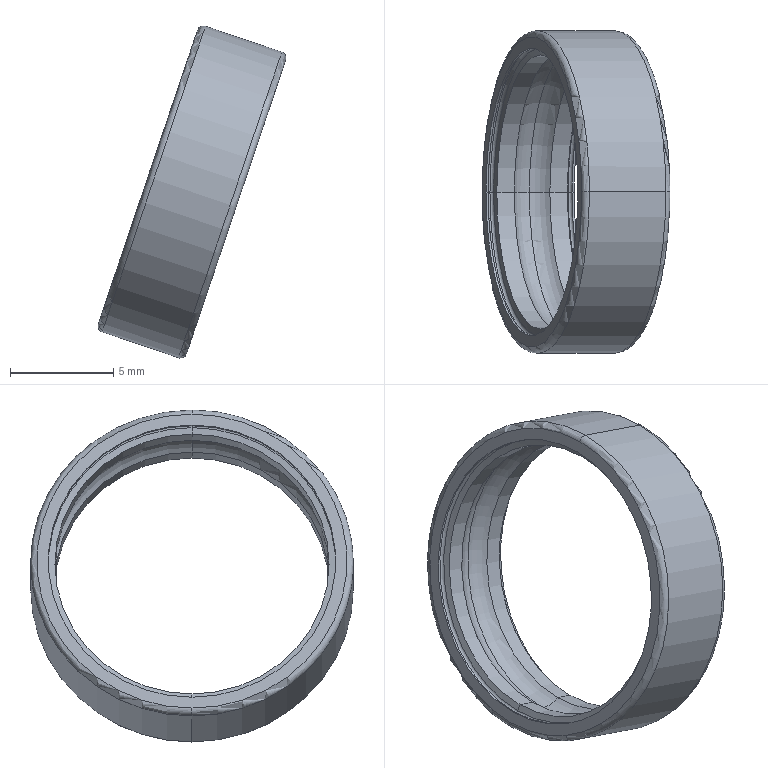Part | STEP file | 2026.6.15-Main Assembly图.sldasm-Part-183 | 1 solid | 32 faces | box 9.094 x 15.6 x 16.059 mm | volume 200.393 mm3 | torus 16 | cylinder 10 | cone 4 | plane 2 | commonest cylinder face diameters 13.26 x4 13.89 x4 15.6 x2
STEP:
#1=CARTESIAN_POINT('',(-1651.759,1424.264,3250.576));
#2=VERTEX_POINT('',#1);
#3=CARTESIAN_POINT('',(-1652.483,1424.264,3251.26));
#4=VERTEX_POINT('',#3);
#5=CARTESIAN_POINT('',(-1652.864,1424.264,3250.132));
#6=DIRECTION('',(0.,-1.,0.));
#7=DIRECTION('',(0.3199,0.,0.9474));
#8=AXIS2_PLACEMENT_3D('',#5,#6,#7);
#9=CIRCLE('',#8,1.191);
#10=EDGE_CURVE('',#2,#4,#9,.T.);
#11=ORIENTED_EDGE('',*,*,#10,.F.);
#12=CARTESIAN_POINT('',(-1656.002,1424.264,3238.013));
#13=VERTEX_POINT('',#12);
#14=CARTESIAN_POINT('',(-1653.88,1424.264,3244.295));
#15=DIRECTION('',(0.9474,0.,-0.3199));
#16=DIRECTION('',(-0.3199,0.,-0.9474));
#17=AXIS2_PLACEMENT_3D('',#14,#15,#16);
#18=CIRCLE('',#17,6.63);
#19=EDGE_CURVE('',#2,#13,#18,.T.);
#20=ORIENTED_EDGE('',*,*,#19,.T.);
#21=CARTESIAN_POINT('',(-1656.992,1424.264,3237.908));
#22=VERTEX_POINT('',#21);
#23=CARTESIAN_POINT('',(-1656.611,1424.264,3239.036));
#24=DIRECTION('',(0.,1.,0.));
#25=DIRECTION('',(-0.3199,0.,-0.9474));
#26=AXIS2_PLACEMENT_3D('',#23,#24,#25);
#27=CIRCLE('',#26,1.191);
#28=EDGE_CURVE('',#13,#22,#27,.T.);
#29=ORIENTED_EDGE('',*,*,#28,.T.);
#30=CARTESIAN_POINT('',(-1654.738,1424.264,3244.584));
#31=DIRECTION('',(0.9474,0.,-0.3199));
#32=DIRECTION('',(-0.3199,0.,-0.9474));
#33=AXIS2_PLACEMENT_3D('',#30,#31,#32);
#34=CIRCLE('',#33,7.047);
#35=EDGE_CURVE('',#4,#22,#34,.T.);
#36=ORIENTED_EDGE('',*,*,#35,.F.);
#37=EDGE_LOOP('',(#11,#20,#29,#36));
#38=FACE_OUTER_BOUND('',#37,.T.);
#39=CARTESIAN_POINT('',(-1654.738,1424.264,3244.584));
#40=DIRECTION('',(0.9474,0.,-0.3199));
#41=DIRECTION('',(-0.3199,0.,-0.9474));
#42=AXIS2_PLACEMENT_3D('',#39,#40,#41);
#43=TOROIDAL_SURFACE('',#42,5.856,1.191);
#44=ADVANCED_FACE('',(#38),#43,.F.);
#45=CARTESIAN_POINT('',(-1654.324,1424.264,3251.442));
#46=VERTEX_POINT('',#45);
#47=CARTESIAN_POINT('',(-1653.474,1424.264,3251.155));
#48=VERTEX_POINT('',#47);
#49=CARTESIAN_POINT('',(-1650.769,1424.264,3250.242));
#50=DIRECTION('',(0.9474,0.,-0.3199));
#51=VECTOR('',#50,1000.);
#52=LINE('',#49,#51);
#53=EDGE_CURVE('',#46,#48,#52,.T.);
#54=ORIENTED_EDGE('',*,*,#53,.F.);
#55=CARTESIAN_POINT('',(-1658.566,1424.264,3238.879));
#56=VERTEX_POINT('',#55);
#57=CARTESIAN_POINT('',(-1656.445,1424.264,3245.161));
#58=DIRECTION('',(-0.9474,0.,0.3199));
#59=DIRECTION('',(0.3199,0.,0.9474));
#60=AXIS2_PLACEMENT_3D('',#57,#58,#59);
#61=CIRCLE('',#60,6.63);
#62=EDGE_CURVE('',#46,#56,#61,.T.);
#63=ORIENTED_EDGE('',*,*,#62,.T.);
#64=CARTESIAN_POINT('',(-1657.716,1424.264,3238.592));
#65=VERTEX_POINT('',#64);
#66=CARTESIAN_POINT('',(-1655.011,1424.264,3237.679));
#67=DIRECTION('',(0.9474,0.,-0.3199));
#68=VECTOR('',#67,1000.);
#69=LINE('',#66,#68);
#70=EDGE_CURVE('',#56,#65,#69,.T.);
#71=ORIENTED_EDGE('',*,*,#70,.T.);
#72=CARTESIAN_POINT('',(-1655.595,1424.264,3244.873));
#73=DIRECTION('',(-0.9474,0.,0.3199));
#74=DIRECTION('',(-0.3199,0.,-0.9474));
#75=AXIS2_PLACEMENT_3D('',#72,#73,#74);
#76=CIRCLE('',#75,6.63);
#77=EDGE_CURVE('',#48,#65,#76,.T.);
#78=ORIENTED_EDGE('',*,*,#77,.F.);
#79=EDGE_LOOP('',(#54,#63,#71,#78));
#80=FACE_OUTER_BOUND('',#79,.T.);
#81=CARTESIAN_POINT('',(-1652.89,1424.264,3243.96));
#82=DIRECTION('',(0.9474,0.,-0.3199));
#83=DIRECTION('',(0.3199,0.,0.9474));
#84=AXIS2_PLACEMENT_3D('',#81,#82,#83);
#85=CYLINDRICAL_SURFACE('',#84,6.63);
#86=ADVANCED_FACE('',(#80),#85,.F.);
#87=CARTESIAN_POINT('',(-1650.909,1424.264,3250.289));
#88=VERTEX_POINT('',#87);
#89=CARTESIAN_POINT('',(-1650.769,1424.264,3250.242));
#90=DIRECTION('',(0.9474,0.,-0.3199));
#91=VECTOR('',#90,1000.);
#92=LINE('',#89,#91);
#93=EDGE_CURVE('',#2,#88,#92,.T.);
#94=ORIENTED_EDGE('',*,*,#93,.F.);
#95=CARTESIAN_POINT('',(-1653.88,1424.264,3244.295));
#96=DIRECTION('',(0.9474,0.,-0.3199));
#97=DIRECTION('',(-0.3199,0.,-0.9474));
#98=AXIS2_PLACEMENT_3D('',#95,#96,#97);
#99=CIRCLE('',#98,6.63);
#100=EDGE_CURVE('',#13,#2,#99,.T.);
#101=ORIENTED_EDGE('',*,*,#100,.F.);
#102=CARTESIAN_POINT('',(-1655.152,1424.264,3237.726));
#103=VERTEX_POINT('',#102);
#104=CARTESIAN_POINT('',(-1655.011,1424.264,3237.679));
#105=DIRECTION('',(0.9474,0.,-0.3199));
#106=VECTOR('',#105,1000.);
#107=LINE('',#104,#106);
#108=EDGE_CURVE('',#13,#103,#107,.T.);
#109=ORIENTED_EDGE('',*,*,#108,.T.);
#110=CARTESIAN_POINT('',(-1653.03,1430.894,3244.007));
#111=VERTEX_POINT('',#110);
#112=CARTESIAN_POINT('',(-1653.03,1424.264,3244.007));
#113=DIRECTION('',(0.9474,0.,-0.3199));
#114=DIRECTION('',(-0.3199,0.,-0.9474));
#115=AXIS2_PLACEMENT_3D('',#112,#113,#114);
#116=CIRCLE('',#115,6.63);
#117=EDGE_CURVE('',#103,#111,#116,.T.);
#118=ORIENTED_EDGE('',*,*,#117,.T.);
#119=CARTESIAN_POINT('',(-1653.03,1424.264,3244.007));
#120=DIRECTION('',(0.9474,0.,-0.3199));
#121=DIRECTION('',(-0.3199,0.,-0.9474));
#122=AXIS2_PLACEMENT_3D('',#119,#120,#121);
#123=CIRCLE('',#122,6.63);
#124=EDGE_CURVE('',#111,#88,#123,.T.);
#125=ORIENTED_EDGE('',*,*,#124,.T.);
#126=EDGE_LOOP('',(#94,#101,#109,#118,#125));
#127=FACE_OUTER_BOUND('',#126,.T.);
#128=CARTESIAN_POINT('',(-1652.89,1424.264,3243.96));
#129=DIRECTION('',(0.9474,0.,-0.3199));
#130=DIRECTION('',(0.3199,0.,0.9474));
#131=AXIS2_PLACEMENT_3D('',#128,#129,#130);
#132=CYLINDRICAL_SURFACE('',#131,6.63);
#133=ADVANCED_FACE('',(#127),#132,.F.);
#134=CARTESIAN_POINT('',(-1658.719,1424.264,3238.598));
#135=VERTEX_POINT('',#134);
#136=CARTESIAN_POINT('',(-1658.719,1424.264,3238.598));
#137=DIRECTION('',(0.4796,0.,0.8775));
#138=VECTOR('',#137,1000.);
#139=LINE('',#136,#138);
#140=EDGE_CURVE('',#135,#56,#139,.T.);
#141=ORIENTED_EDGE('',*,*,#140,.T.);
#142=ORIENTED_EDGE('',*,*,#62,.F.);
#143=CARTESIAN_POINT('',(-1654.275,1424.264,3251.758));
#144=VERTEX_POINT('',#143);
#145=CARTESIAN_POINT('',(-1654.275,1424.264,3251.758));
#146=DIRECTION('',(-0.1506,0.,-0.9886));
#147=VECTOR('',#146,1000.);
#148=LINE('',#145,#147);
#149=EDGE_CURVE('',#144,#46,#148,.T.);
#150=ORIENTED_EDGE('',*,*,#149,.F.);
#151=CARTESIAN_POINT('',(-1656.497,1424.264,3245.178));
#152=DIRECTION('',(-0.9474,0.,0.3199));
#153=DIRECTION('',(-0.3199,0.,-0.9474));
#154=AXIS2_PLACEMENT_3D('',#151,#152,#153);
#155=CIRCLE('',#154,6.945);
#156=EDGE_CURVE('',#144,#135,#155,.T.);
#157=ORIENTED_EDGE('',*,*,#156,.T.);
#158=EDGE_LOOP('',(#141,#142,#150,#157));
#159=FACE_OUTER_BOUND('',#158,.T.);
#160=CARTESIAN_POINT('',(-1656.497,1424.264,3245.178));
#161=DIRECTION('',(-0.9474,0.,0.3199));
#162=DIRECTION('',(-0.3199,0.,-0.9474));
#163=AXIS2_PLACEMENT_3D('',#160,#161,#162);
#164=CONICAL_SURFACE('',#163,6.945,1.396);
#165=ADVANCED_FACE('',(#159),#164,.F.);
#166=CARTESIAN_POINT('',(-1652.978,1417.319,3243.99));
#167=VERTEX_POINT('',#166);
#168=CARTESIAN_POINT('',(-1653.03,1417.634,3244.007));
#169=VERTEX_POINT('',#168);
#170=CARTESIAN_POINT('',(-1652.978,1417.319,3243.99));
#171=DIRECTION('',(-0.1645,0.9848,0.05556));
#172=VECTOR('',#171,1000.);
#173=LINE('',#170,#172);
#174=EDGE_CURVE('',#167,#169,#173,.T.);
#175=ORIENTED_EDGE('',*,*,#174,.T.);
#176=CARTESIAN_POINT('',(-1653.03,1424.264,3244.007));
#177=DIRECTION('',(0.9474,0.,-0.3199));
#178=DIRECTION('',(-0.3199,0.,-0.9474));
#179=AXIS2_PLACEMENT_3D('',#176,#177,#178);
#180=CIRCLE('',#179,6.63);
#181=EDGE_CURVE('',#88,#169,#180,.T.);
#182=ORIENTED_EDGE('',*,*,#181,.F.);
#183=ORIENTED_EDGE('',*,*,#124,.F.);
#184=CARTESIAN_POINT('',(-1652.978,1431.209,3243.99));
#185=VERTEX_POINT('',#184);
#186=CARTESIAN_POINT('',(-1652.978,1431.209,3243.99));
#187=DIRECTION('',(-0.1645,-0.9848,0.05556));
#188=VECTOR('',#187,1000.);
#189=LINE('',#186,#188);
#190=EDGE_CURVE('',#185,#111,#189,.T.);
#191=ORIENTED_EDGE('',*,*,#190,.F.);
#192=CARTESIAN_POINT('',(-1650.756,1424.264,3250.57));
#193=VERTEX_POINT('',#192);
#194=CARTESIAN_POINT('',(-1652.978,1424.264,3243.99));
#195=DIRECTION('',(0.9474,0.,-0.3199));
#196=DIRECTION('',(-0.3199,0.,-0.9474));
#197=AXIS2_PLACEMENT_3D('',#194,#195,#196);
#198=CIRCLE('',#197,6.945);
#199=EDGE_CURVE('',#185,#193,#198,.T.);
#200=ORIENTED_EDGE('',*,*,#199,.T.);
#201=CARTESIAN_POINT('',(-1652.978,1424.264,3243.99));
#202=DIRECTION('',(0.9474,0.,-0.3199));
#203=DIRECTION('',(-0.3199,0.,-0.9474));
#204=AXIS2_PLACEMENT_3D('',#201,#202,#203);
#205=CIRCLE('',#204,6.945);
#206=EDGE_CURVE('',#193,#167,#205,.T.);
#207=ORIENTED_EDGE('',*,*,#206,.T.);
#208=EDGE_LOOP('',(#175,#182,#183,#191,#200,#207));
#209=FACE_OUTER_BOUND('',#208,.T.);
#210=CARTESIAN_POINT('',(-1652.978,1424.264,3243.99));
#211=DIRECTION('',(0.9474,0.,-0.3199));
#212=DIRECTION('',(0.,-1.,0.));
#213=AXIS2_PLACEMENT_3D('',#210,#211,#212);
#214=CONICAL_SURFACE('',#213,6.945,1.396);
#215=ADVANCED_FACE('',(#209),#214,.F.);
#216=CARTESIAN_POINT('',(-1654.364,1424.264,3251.937));
#217=VERTEX_POINT('',#216);
#218=CARTESIAN_POINT('',(-1654.409,1424.264,3251.803));
#219=DIRECTION('',(0.,-1.,0.));
#220=DIRECTION('',(0.3199,0.,0.9474));
#221=AXIS2_PLACEMENT_3D('',#218,#219,#220);
#222=CIRCLE('',#221,0.1413);
#223=EDGE_CURVE('',#144,#217,#222,.T.);
#224=ORIENTED_EDGE('',*,*,#223,.F.);
#225=CARTESIAN_POINT('',(-1656.497,1424.264,3245.178));
#226=DIRECTION('',(-0.9474,0.,0.3199));
#227=DIRECTION('',(-0.3199,0.,-0.9474));
#228=AXIS2_PLACEMENT_3D('',#225,#226,#227);
#229=CIRCLE('',#228,6.945);
#230=EDGE_CURVE('',#135,#144,#229,.T.);
#231=ORIENTED_EDGE('',*,*,#230,.F.);
#232=CARTESIAN_POINT('',(-1658.898,1424.264,3238.51));
#233=VERTEX_POINT('',#232);
#234=CARTESIAN_POINT('',(-1658.853,1424.264,3238.644));
#235=DIRECTION('',(0.,1.,0.));
#236=DIRECTION('',(-0.3199,0.,-0.9474));
#237=AXIS2_PLACEMENT_3D('',#234,#235,#236);
#238=CIRCLE('',#237,0.1413);
#239=EDGE_CURVE('',#135,#233,#238,.T.);
#240=ORIENTED_EDGE('',*,*,#239,.T.);
#241=CARTESIAN_POINT('',(-1656.631,1424.264,3245.224));
#242=DIRECTION('',(0.9474,0.,-0.3199));
#243=DIRECTION('',(-0.3199,0.,-0.9474));
#244=AXIS2_PLACEMENT_3D('',#241,#242,#243);
#245=CIRCLE('',#244,7.086);
#246=EDGE_CURVE('',#217,#233,#245,.T.);
#247=ORIENTED_EDGE('',*,*,#246,.F.);
#248=EDGE_LOOP('',(#224,#231,#240,#247));
#249=FACE_OUTER_BOUND('',#248,.T.);
#250=CARTESIAN_POINT('',(-1656.631,1424.264,3245.224));
#251=DIRECTION('',(0.9474,0.,-0.3199));
#252=DIRECTION('',(-0.3199,0.,-0.9474));
#253=AXIS2_PLACEMENT_3D('',#250,#251,#252);
#254=TOROIDAL_SURFACE('',#253,6.945,0.1413);
#255=ADVANCED_FACE('',(#249),#254,.F.);
#256=CARTESIAN_POINT('',(-1650.488,1424.264,3250.479));
#257=VERTEX_POINT('',#256);
#258=CARTESIAN_POINT('',(-1650.577,1424.264,3250.658));
#259=VERTEX_POINT('',#258);
#260=CARTESIAN_POINT('',(-1650.622,1424.264,3250.524));
#261=DIRECTION('',(0.,-1.,0.));
#262=DIRECTION('',(0.3199,0.,0.9474));
#263=AXIS2_PLACEMENT_3D('',#260,#261,#262);
#264=CIRCLE('',#263,0.1413);
#265=EDGE_CURVE('',#257,#259,#264,.T.);
#266=ORIENTED_EDGE('',*,*,#265,.F.);
#267=CARTESIAN_POINT('',(-1654.932,1424.264,3237.319));
#268=VERTEX_POINT('',#267);
#269=CARTESIAN_POINT('',(-1652.71,1424.264,3243.899));
#270=DIRECTION('',(0.9474,0.,-0.3199));
#271=DIRECTION('',(-0.3199,0.,-0.9474));
#272=AXIS2_PLACEMENT_3D('',#269,#270,#271);
#273=CIRCLE('',#272,6.945);
#274=EDGE_CURVE('',#257,#268,#273,.T.);
#275=ORIENTED_EDGE('',*,*,#274,.T.);
#276=CARTESIAN_POINT('',(-1655.111,1424.264,3237.231));
#277=VERTEX_POINT('',#276);
#278=CARTESIAN_POINT('',(-1655.066,1424.264,3237.365));
#279=DIRECTION('',(0.,1.,0.));
#280=DIRECTION('',(-0.3199,0.,-0.9474));
#281=AXIS2_PLACEMENT_3D('',#278,#279,#280);
#282=CIRCLE('',#281,0.1413);
#283=EDGE_CURVE('',#268,#277,#282,.T.);
#284=ORIENTED_EDGE('',*,*,#283,.T.);
#285=CARTESIAN_POINT('',(-1652.844,1424.264,3243.944));
#286=DIRECTION('',(0.9474,0.,-0.3199));
#287=DIRECTION('',(-0.3199,0.,-0.9474));
#288=AXIS2_PLACEMENT_3D('',#285,#286,#287);
#289=CIRCLE('',#288,7.086);
#290=EDGE_CURVE('',#259,#277,#289,.T.);
#291=ORIENTED_EDGE('',*,*,#290,.F.);
#292=EDGE_LOOP('',(#266,#275,#284,#291));
#293=FACE_OUTER_BOUND('',#292,.T.);
#294=CARTESIAN_POINT('',(-1652.844,1424.264,3243.944));
#295=DIRECTION('',(0.9474,0.,-0.3199));
#296=DIRECTION('',(-0.3199,0.,-0.9474));
#297=AXIS2_PLACEMENT_3D('',#294,#295,#296);
#298=TOROIDAL_SURFACE('',#297,6.945,0.1413);
#299=ADVANCED_FACE('',(#293),#298,.F.);
#300=CARTESIAN_POINT('',(-1654.647,1424.264,3251.884));
#301=VERTEX_POINT('',#300);
#302=CARTESIAN_POINT('',(-1654.543,1424.264,3251.849));
#303=VERTEX_POINT('',#302);
#304=CARTESIAN_POINT('',(-1650.668,1424.264,3250.54));
#305=DIRECTION('',(0.9474,0.,-0.3199));
#306=VECTOR('',#305,1000.);
#307=LINE('',#304,#306);
#308=EDGE_CURVE('',#301,#303,#307,.T.);
#309=ORIENTED_EDGE('',*,*,#308,.F.);
#310=CARTESIAN_POINT('',(-1659.091,1424.264,3238.724));
#311=VERTEX_POINT('',#310);
#312=CARTESIAN_POINT('',(-1656.869,1424.264,3245.304));
#313=DIRECTION('',(0.9474,0.,-0.3199));
#314=DIRECTION('',(-0.3199,0.,-0.9474));
#315=AXIS2_PLACEMENT_3D('',#312,#313,#314);
#316=CIRCLE('',#315,6.945);
#317=EDGE_CURVE('',#311,#301,#316,.T.);
#318=ORIENTED_EDGE('',*,*,#317,.F.);
#319=CARTESIAN_POINT('',(-1658.987,1424.264,3238.689));
#320=VERTEX_POINT('',#319);
#321=CARTESIAN_POINT('',(-1655.112,1424.264,3237.38));
#322=DIRECTION('',(0.9474,0.,-0.3199));
#323=VECTOR('',#322,1000.);
#324=LINE('',#321,#323);
#325=EDGE_CURVE('',#311,#320,#324,.T.);
#326=ORIENTED_EDGE('',*,*,#325,.T.);
#327=CARTESIAN_POINT('',(-1656.765,1424.264,3245.269));
#328=DIRECTION('',(-0.9474,0.,0.3199));
#329=DIRECTION('',(-0.3199,0.,-0.9474));
#330=AXIS2_PLACEMENT_3D('',#327,#328,#329);
#331=CIRCLE('',#330,6.945);
#332=EDGE_CURVE('',#303,#320,#331,.T.);
#333=ORIENTED_EDGE('',*,*,#332,.F.);
#334=EDGE_LOOP('',(#309,#318,#326,#333));
#335=FACE_OUTER_BOUND('',#334,.T.);
#336=CARTESIAN_POINT('',(-1652.89,1424.264,3243.96));
#337=DIRECTION('',(0.9474,0.,-0.3199));
#338=DIRECTION('',(0.3199,0.,0.9474));
#339=AXIS2_PLACEMENT_3D('',#336,#337,#338);
#340=CYLINDRICAL_SURFACE('',#339,6.945);
#341=ADVANCED_FACE('',(#335),#340,.F.);
#342=CARTESIAN_POINT('',(-1650.384,1424.264,3250.444));
#343=VERTEX_POINT('',#342);
#344=CARTESIAN_POINT('',(-1650.668,1424.264,3250.54));
#345=DIRECTION('',(0.9474,0.,-0.3199));
#346=VECTOR('',#345,1000.);
#347=LINE('',#344,#346);
#348=EDGE_CURVE('',#257,#343,#347,.T.);
#349=ORIENTED_EDGE('',*,*,#348,.F.);
#350=CARTESIAN_POINT('',(-1652.71,1424.264,3243.899));
#351=DIRECTION('',(0.9474,0.,-0.3199));
#352=DIRECTION('',(-0.3199,0.,-0.9474));
#353=AXIS2_PLACEMENT_3D('',#350,#351,#352);
#354=CIRCLE('',#353,6.945);
#355=EDGE_CURVE('',#268,#257,#354,.T.);
#356=ORIENTED_EDGE('',*,*,#355,.F.);
#357=CARTESIAN_POINT('',(-1654.828,1424.264,3237.284));
#358=VERTEX_POINT('',#357);
#359=CARTESIAN_POINT('',(-1655.112,1424.264,3237.38));
#360=DIRECTION('',(0.9474,0.,-0.3199));
#361=VECTOR('',#360,1000.);
#362=LINE('',#359,#361);
#363=EDGE_CURVE('',#268,#358,#362,.T.);
#364=ORIENTED_EDGE('',*,*,#363,.T.);
#365=CARTESIAN_POINT('',(-1652.606,1424.264,3243.864));
#366=DIRECTION('',(-0.9474,0.,0.3199));
#367=DIRECTION('',(-0.3199,0.,-0.9474));
#368=AXIS2_PLACEMENT_3D('',#365,#366,#367);
#369=CIRCLE('',#368,6.945);
#370=EDGE_CURVE('',#343,#358,#369,.T.);
#371=ORIENTED_EDGE('',*,*,#370,.F.);
#372=EDGE_LOOP('',(#349,#356,#364,#371));
#373=FACE_OUTER_BOUND('',#372,.T.);
#374=CARTESIAN_POINT('',(-1652.89,1424.264,3243.96));
#375=DIRECTION('',(0.9474,0.,-0.3199));
#376=DIRECTION('',(0.3199,0.,0.9474));
#377=AXIS2_PLACEMENT_3D('',#374,#375,#376);
#378=CYLINDRICAL_SURFACE('',#377,6.945);
#379=ADVANCED_FACE('',(#373),#378,.F.);
#380=CARTESIAN_POINT('',(-1659.269,1424.264,3238.198));
#381=VERTEX_POINT('',#380);
#382=CARTESIAN_POINT('',(-1654.47,1424.264,3252.41));
#383=VERTEX_POINT('',#382);
#384=CARTESIAN_POINT('',(-1656.869,1424.264,3245.304));
#385=DIRECTION('',(0.9474,0.,-0.3199));
#386=DIRECTION('',(-0.3199,0.,-0.9474));
#387=AXIS2_PLACEMENT_3D('',#384,#385,#386);
#388=CIRCLE('',#387,7.5);
#389=EDGE_CURVE('',#381,#383,#388,.T.);
#390=ORIENTED_EDGE('',*,*,#389,.F.);
#391=CARTESIAN_POINT('',(-1656.869,1424.264,3245.304));
#392=DIRECTION('',(0.9474,0.,-0.3199));
#393=DIRECTION('',(-0.3199,0.,-0.9474));
#394=AXIS2_PLACEMENT_3D('',#391,#392,#393);
#395=CIRCLE('',#394,7.5);
#396=EDGE_CURVE('',#383,#381,#395,.T.);
#397=ORIENTED_EDGE('',*,*,#396,.F.);
#398=EDGE_LOOP('',(#390,#397));
#399=FACE_OUTER_BOUND('',#398,.T.);
#400=ORIENTED_EDGE('',*,*,#317,.T.);
#401=CARTESIAN_POINT('',(-1656.869,1424.264,3245.304));
#402=DIRECTION('',(0.9474,0.,-0.3199));
#403=DIRECTION('',(-0.3199,0.,-0.9474));
#404=AXIS2_PLACEMENT_3D('',#401,#402,#403);
#405=CIRCLE('',#404,6.945);
#406=EDGE_CURVE('',#301,#311,#405,.T.);
#407=ORIENTED_EDGE('',*,*,#406,.T.);
#408=EDGE_LOOP('',(#400,#407));
#409=FACE_BOUND('',#408,.T.);
#410=CARTESIAN_POINT('',(-1656.869,1431.764,3245.304));
#411=DIRECTION('',(-0.9474,0.,0.3199));
#412=DIRECTION('',(0.,1.,0.));
#413=AXIS2_PLACEMENT_3D('',#410,#411,#412);
#414=PLANE('',#413);
#415=ADVANCED_FACE('',(#399,#409),#414,.T.);
#416=CARTESIAN_POINT('',(-1650.206,1424.264,3250.97));
#417=VERTEX_POINT('',#416);
#418=CARTESIAN_POINT('',(-1655.005,1424.264,3236.758));
#419=VERTEX_POINT('',#418);
#420=CARTESIAN_POINT('',(-1652.606,1424.264,3243.864));
#421=DIRECTION('',(-0.9474,0.,0.3199));
#422=DIRECTION('',(0.3199,0.,0.9474));
#423=AXIS2_PLACEMENT_3D('',#420,#421,#422);
#424=CIRCLE('',#423,7.5);
#425=EDGE_CURVE('',#417,#419,#424,.T.);
#426=ORIENTED_EDGE('',*,*,#425,.F.);
#427=CARTESIAN_POINT('',(-1652.606,1424.264,3243.864));
#428=DIRECTION('',(-0.9474,0.,0.3199));
#429=DIRECTION('',(0.3199,0.,0.9474));
#430=AXIS2_PLACEMENT_3D('',#427,#428,#429);
#431=CIRCLE('',#430,7.5);
#432=EDGE_CURVE('',#419,#417,#431,.T.);
#433=ORIENTED_EDGE('',*,*,#432,.F.);
#434=EDGE_LOOP('',(#426,#433));
#435=FACE_OUTER_BOUND('',#434,.T.);
#436=CARTESIAN_POINT('',(-1652.606,1424.264,3243.864));
#437=DIRECTION('',(-0.9474,0.,0.3199));
#438=DIRECTION('',(-0.3199,0.,-0.9474));
#439=AXIS2_PLACEMENT_3D('',#436,#437,#438);
#440=CIRCLE('',#439,6.945);
#441=EDGE_CURVE('',#358,#343,#440,.T.);
#442=ORIENTED_EDGE('',*,*,#441,.T.);
#443=ORIENTED_EDGE('',*,*,#370,.T.);
#444=EDGE_LOOP('',(#442,#443));
#445=FACE_BOUND('',#444,.T.);
#446=CARTESIAN_POINT('',(-1652.606,1431.209,3243.864));
#447=DIRECTION('',(0.9474,0.,-0.3199));
#448=DIRECTION('',(0.,-1.,0.));
#449=AXIS2_PLACEMENT_3D('',#446,#447,#448);
#450=PLANE('',#449);
#451=ADVANCED_FACE('',(#435,#445),#450,.T.);
#452=CARTESIAN_POINT('',(-1654.089,1424.264,3252.598));
#453=VERTEX_POINT('',#452);
#454=CARTESIAN_POINT('',(-1654.185,1424.264,3252.314));
#455=DIRECTION('',(0.,-1.,0.));
#456=DIRECTION('',(0.3199,0.,0.9474));
#457=AXIS2_PLACEMENT_3D('',#454,#455,#456);
#458=CIRCLE('',#457,0.3);
#459=EDGE_CURVE('',#453,#383,#458,.T.);
#460=ORIENTED_EDGE('',*,*,#459,.F.);
#461=CARTESIAN_POINT('',(-1659.081,1424.264,3237.818));
#462=VERTEX_POINT('',#461);
#463=CARTESIAN_POINT('',(-1656.585,1424.264,3245.208));
#464=DIRECTION('',(0.9474,0.,-0.3199));
#465=DIRECTION('',(-0.3199,0.,-0.9474));
#466=AXIS2_PLACEMENT_3D('',#463,#464,#465);
#467=CIRCLE('',#466,7.8);
#468=EDGE_CURVE('',#462,#453,#467,.T.);
#469=ORIENTED_EDGE('',*,*,#468,.F.);
#470=CARTESIAN_POINT('',(-1658.985,1424.264,3238.102));
#471=DIRECTION('',(0.,1.,0.));
#472=DIRECTION('',(-0.3199,0.,-0.9474));
#473=AXIS2_PLACEMENT_3D('',#470,#471,#472);
#474=CIRCLE('',#473,0.3);
#475=EDGE_CURVE('',#462,#381,#474,.T.);
#476=ORIENTED_EDGE('',*,*,#475,.T.);
#477=ORIENTED_EDGE('',*,*,#389,.T.);
#478=EDGE_LOOP('',(#460,#469,#476,#477));
#479=FACE_OUTER_BOUND('',#478,.T.);
#480=CARTESIAN_POINT('',(-1656.585,1424.264,3245.208));
#481=DIRECTION('',(0.9474,0.,-0.3199));
#482=DIRECTION('',(-0.3199,0.,-0.9474));
#483=AXIS2_PLACEMENT_3D('',#480,#481,#482);
#484=TOROIDAL_SURFACE('',#483,7.5,0.3);
#485=ADVANCED_FACE('',(#479),#484,.T.);
#486=CARTESIAN_POINT('',(-1650.394,1424.264,3251.35));
#487=VERTEX_POINT('',#486);
#488=CARTESIAN_POINT('',(-1650.49,1424.264,3251.066));
#489=DIRECTION('',(0.,-1.,0.));
#490=DIRECTION('',(0.3199,0.,0.9474));
#491=AXIS2_PLACEMENT_3D('',#488,#489,#490);
#492=CIRCLE('',#491,0.3);
#493=EDGE_CURVE('',#417,#487,#492,.T.);
#494=ORIENTED_EDGE('',*,*,#493,.F.);
#495=ORIENTED_EDGE('',*,*,#425,.T.);
#496=CARTESIAN_POINT('',(-1655.386,1424.264,3236.57));
#497=VERTEX_POINT('',#496);
#498=CARTESIAN_POINT('',(-1655.29,1424.264,3236.854));
#499=DIRECTION('',(0.,1.,0.));
#500=DIRECTION('',(-0.3199,0.,-0.9474));
#501=AXIS2_PLACEMENT_3D('',#498,#499,#500);
#502=CIRCLE('',#501,0.3);
#503=EDGE_CURVE('',#419,#497,#502,.T.);
#504=ORIENTED_EDGE('',*,*,#503,.T.);
#505=CARTESIAN_POINT('',(-1652.89,1424.264,3243.96));
#506=DIRECTION('',(-0.9474,0.,0.3199));
#507=DIRECTION('',(-0.3199,0.,-0.9474));
#508=AXIS2_PLACEMENT_3D('',#505,#506,#507);
#509=CIRCLE('',#508,7.8);
#510=EDGE_CURVE('',#487,#497,#509,.T.);
#511=ORIENTED_EDGE('',*,*,#510,.F.);
#512=EDGE_LOOP('',(#494,#495,#504,#511));
#513=FACE_OUTER_BOUND('',#512,.T.);
#514=CARTESIAN_POINT('',(-1652.89,1424.264,3243.96));
#515=DIRECTION('',(0.9474,0.,-0.3199));
#516=DIRECTION('',(-0.3199,0.,-0.9474));
#517=AXIS2_PLACEMENT_3D('',#514,#515,#516);
#518=TOROIDAL_SURFACE('',#517,7.5,0.3);
#519=ADVANCED_FACE('',(#513),#518,.T.);
#520=CARTESIAN_POINT('',(-1650.394,1424.264,3251.35));
#521=DIRECTION('',(0.9474,0.,-0.3199));
#522=VECTOR('',#521,1000.);
#523=LINE('',#520,#522);
#524=EDGE_CURVE('',#453,#487,#523,.T.);
#525=ORIENTED_EDGE('',*,*,#524,.F.);
#526=CARTESIAN_POINT('',(-1656.585,1424.264,3245.208));
#527=DIRECTION('',(0.9474,0.,-0.3199));
#528=DIRECTION('',(-0.3199,0.,-0.9474));
#529=AXIS2_PLACEMENT_3D('',#526,#527,#528);
#530=CIRCLE('',#529,7.8);
#531=EDGE_CURVE('',#453,#462,#530,.T.);
#532=ORIENTED_EDGE('',*,*,#531,.T.);
#533=CARTESIAN_POINT('',(-1655.386,1424.264,3236.57));
#534=DIRECTION('',(0.9474,0.,-0.3199));
#535=VECTOR('',#534,1000.);
#536=LINE('',#533,#535);
#537=EDGE_CURVE('',#462,#497,#536,.T.);
#538=ORIENTED_EDGE('',*,*,#537,.T.);
#539=CARTESIAN_POINT('',(-1652.89,1424.264,3243.96));
#540=DIRECTION('',(-0.9474,0.,0.3199));
#541=DIRECTION('',(-0.3199,0.,-0.9474));
#542=AXIS2_PLACEMENT_3D('',#539,#540,#541);
#543=CIRCLE('',#542,7.8);
#544=EDGE_CURVE('',#497,#487,#543,.T.);
#545=ORIENTED_EDGE('',*,*,#544,.T.);
#546=EDGE_LOOP('',(#525,#532,#538,#545));
#547=FACE_OUTER_BOUND('',#546,.T.);
#548=CARTESIAN_POINT('',(-1652.89,1424.264,3243.96));
#549=DIRECTION('',(0.9474,0.,-0.3199));
#550=DIRECTION('',(0.3199,0.,0.9474));
#551=AXIS2_PLACEMENT_3D('',#548,#549,#550);
#552=CYLINDRICAL_SURFACE('',#551,7.8);
#553=ADVANCED_FACE('',(#547),#552,.T.);
#554=CARTESIAN_POINT('',(-1652.864,1424.264,3250.132));
#555=DIRECTION('',(0.,-1.,0.));
#556=DIRECTION('',(0.3199,0.,0.9474));
#557=AXIS2_PLACEMENT_3D('',#554,#555,#556);
#558=CIRCLE('',#557,1.191);
#559=EDGE_CURVE('',#4,#48,#558,.T.);
#560=ORIENTED_EDGE('',*,*,#559,.F.);
#561=ORIENTED_EDGE('',*,*,#35,.T.);
#562=CARTESIAN_POINT('',(-1656.611,1424.264,3239.036));
#563=DIRECTION('',(0.,1.,0.));
#564=DIRECTION('',(-0.3199,0.,-0.9474));
#565=AXIS2_PLACEMENT_3D('',#562,#563,#564);
#566=CIRCLE('',#565,1.191);
#567=EDGE_CURVE('',#22,#65,#566,.T.);
#568=ORIENTED_EDGE('',*,*,#567,.T.);
#569=CARTESIAN_POINT('',(-1655.595,1424.264,3244.873));
#570=DIRECTION('',(-0.9474,0.,0.3199));
#571=DIRECTION('',(-0.3199,0.,-0.9474));
#572=AXIS2_PLACEMENT_3D('',#569,#570,#571);
#573=CIRCLE('',#572,6.63);
#574=EDGE_CURVE('',#65,#48,#573,.T.);
#575=ORIENTED_EDGE('',*,*,#574,.T.);
#576=EDGE_LOOP('',(#560,#561,#568,#575));
#577=FACE_OUTER_BOUND('',#576,.T.);
#578=CARTESIAN_POINT('',(-1654.738,1424.264,3244.584));
#579=DIRECTION('',(0.9474,0.,-0.3199));
#580=DIRECTION('',(-0.3199,0.,-0.9474));
#581=AXIS2_PLACEMENT_3D('',#578,#579,#580);
#582=TOROIDAL_SURFACE('',#581,5.856,1.191);
#583=ADVANCED_FACE('',(#577),#582,.F.);
#584=CARTESIAN_POINT('',(-1656.445,1424.264,3245.161));
#585=DIRECTION('',(-0.9474,0.,0.3199));
#586=DIRECTION('',(0.3199,0.,0.9474));
#587=AXIS2_PLACEMENT_3D('',#584,#585,#586);
#588=CIRCLE('',#587,6.63);
#589=EDGE_CURVE('',#56,#46,#588,.T.);
#590=ORIENTED_EDGE('',*,*,#589,.T.);
#591=ORIENTED_EDGE('',*,*,#53,.T.);
#592=ORIENTED_EDGE('',*,*,#574,.F.);
#593=ORIENTED_EDGE('',*,*,#70,.F.);
#594=EDGE_LOOP('',(#590,#591,#592,#593));
#595=FACE_OUTER_BOUND('',#594,.T.);
#596=CARTESIAN_POINT('',(-1652.89,1424.264,3243.96));
#597=DIRECTION('',(0.9474,0.,-0.3199));
#598=DIRECTION('',(0.3199,0.,0.9474));
#599=AXIS2_PLACEMENT_3D('',#596,#597,#598);
#600=CYLINDRICAL_SURFACE('',#599,6.63);
#601=ADVANCED_FACE('',(#595),#600,.F.);
#602=ORIENTED_EDGE('',*,*,#19,.F.);
#603=ORIENTED_EDGE('',*,*,#93,.T.);
#604=ORIENTED_EDGE('',*,*,#181,.T.);
#605=CARTESIAN_POINT('',(-1653.03,1424.264,3244.007));
#606=DIRECTION('',(0.9474,0.,-0.3199));
#607=DIRECTION('',(-0.3199,0.,-0.9474));
#608=AXIS2_PLACEMENT_3D('',#605,#606,#607);
#609=CIRCLE('',#608,6.63);
#610=EDGE_CURVE('',#169,#103,#609,.T.);
#611=ORIENTED_EDGE('',*,*,#610,.T.);
#612=ORIENTED_EDGE('',*,*,#108,.F.);
#613=EDGE_LOOP('',(#602,#603,#604,#611,#612));
#614=FACE_OUTER_BOUND('',#613,.T.);
#615=CARTESIAN_POINT('',(-1652.89,1424.264,3243.96));
#616=DIRECTION('',(0.9474,0.,-0.3199));
#617=DIRECTION('',(0.3199,0.,0.9474));
#618=AXIS2_PLACEMENT_3D('',#615,#616,#617);
#619=CYLINDRICAL_SURFACE('',#618,6.63);
#620=ADVANCED_FACE('',(#614),#619,.F.);
#621=ORIENTED_EDGE('',*,*,#589,.F.);
#622=ORIENTED_EDGE('',*,*,#140,.F.);
#623=ORIENTED_EDGE('',*,*,#230,.T.);
#624=ORIENTED_EDGE('',*,*,#149,.T.);
#625=EDGE_LOOP('',(#621,#622,#623,#624));
#626=FACE_OUTER_BOUND('',#625,.T.);
#627=CARTESIAN_POINT('',(-1656.497,1424.264,3245.178));
#628=DIRECTION('',(-0.9474,0.,0.3199));
#629=DIRECTION('',(-0.3199,0.,-0.9474));
#630=AXIS2_PLACEMENT_3D('',#627,#628,#629);
#631=CONICAL_SURFACE('',#630,6.945,1.396);
#632=ADVANCED_FACE('',(#626),#631,.F.);
#633=ORIENTED_EDGE('',*,*,#610,.F.);
#634=ORIENTED_EDGE('',*,*,#174,.F.);
#635=CARTESIAN_POINT('',(-1655.2,1424.264,3237.41));
#636=VERTEX_POINT('',#635);
#637=CARTESIAN_POINT('',(-1652.978,1424.264,3243.99));
#638=DIRECTION('',(0.9474,0.,-0.3199));
#639=DIRECTION('',(-0.3199,0.,-0.9474));
#640=AXIS2_PLACEMENT_3D('',#637,#638,#639);
#641=CIRCLE('',#640,6.945);
#642=EDGE_CURVE('',#167,#636,#641,.T.);
#643=ORIENTED_EDGE('',*,*,#642,.T.);
#644=CARTESIAN_POINT('',(-1652.978,1424.264,3243.99));
#645=DIRECTION('',(0.9474,0.,-0.3199));
#646=DIRECTION('',(-0.3199,0.,-0.9474));
#647=AXIS2_PLACEMENT_3D('',#644,#645,#646);
#648=CIRCLE('',#647,6.945);
#649=EDGE_CURVE('',#636,#185,#648,.T.);
#650=ORIENTED_EDGE('',*,*,#649,.T.);
#651=ORIENTED_EDGE('',*,*,#190,.T.);
#652=ORIENTED_EDGE('',*,*,#117,.F.);
#653=EDGE_LOOP('',(#633,#634,#643,#650,#651,#652));
#654=FACE_OUTER_BOUND('',#653,.T.);
#655=CARTESIAN_POINT('',(-1652.978,1424.264,3243.99));
#656=DIRECTION('',(0.9474,0.,-0.3199));
#657=DIRECTION('',(0.,-1.,0.));
#658=AXIS2_PLACEMENT_3D('',#655,#656,#657);
#659=CONICAL_SURFACE('',#658,6.945,1.396);
#660=ADVANCED_FACE('',(#654),#659,.F.);
#661=CARTESIAN_POINT('',(-1654.409,1424.264,3251.803));
#662=DIRECTION('',(0.,-1.,0.));
#663=DIRECTION('',(0.3199,0.,0.9474));
#664=AXIS2_PLACEMENT_3D('',#661,#662,#663);
#665=CIRCLE('',#664,0.1413);
#666=EDGE_CURVE('',#217,#303,#665,.T.);
#667=ORIENTED_EDGE('',*,*,#666,.F.);
#668=ORIENTED_EDGE('',*,*,#246,.T.);
#669=CARTESIAN_POINT('',(-1658.853,1424.264,3238.644));
#670=DIRECTION('',(0.,1.,0.));
#671=DIRECTION('',(-0.3199,0.,-0.9474));
#672=AXIS2_PLACEMENT_3D('',#669,#670,#671);
#673=CIRCLE('',#672,0.1413);
#674=EDGE_CURVE('',#233,#320,#673,.T.);
#675=ORIENTED_EDGE('',*,*,#674,.T.);
#676=CARTESIAN_POINT('',(-1656.765,1424.264,3245.269));
#677=DIRECTION('',(-0.9474,0.,0.3199));
#678=DIRECTION('',(-0.3199,0.,-0.9474));
#679=AXIS2_PLACEMENT_3D('',#676,#677,#678);
#680=CIRCLE('',#679,6.945);
#681=EDGE_CURVE('',#320,#303,#680,.T.);
#682=ORIENTED_EDGE('',*,*,#681,.T.);
#683=EDGE_LOOP('',(#667,#668,#675,#682));
#684=FACE_OUTER_BOUND('',#683,.T.);
#685=CARTESIAN_POINT('',(-1656.631,1424.264,3245.224));
#686=DIRECTION('',(0.9474,0.,-0.3199));
#687=DIRECTION('',(-0.3199,0.,-0.9474));
#688=AXIS2_PLACEMENT_3D('',#685,#686,#687);
#689=TOROIDAL_SURFACE('',#688,6.945,0.1413);
#690=ADVANCED_FACE('',(#684),#689,.F.);
#691=CARTESIAN_POINT('',(-1650.622,1424.264,3250.524));
#692=DIRECTION('',(0.,-1.,0.));
#693=DIRECTION('',(0.3199,0.,0.9474));
#694=AXIS2_PLACEMENT_3D('',#691,#692,#693);
#695=CIRCLE('',#694,0.1413);
#696=EDGE_CURVE('',#259,#193,#695,.T.);
#697=ORIENTED_EDGE('',*,*,#696,.F.);
#698=ORIENTED_EDGE('',*,*,#290,.T.);
#699=CARTESIAN_POINT('',(-1655.066,1424.264,3237.365));
#700=DIRECTION('',(0.,1.,0.));
#701=DIRECTION('',(-0.3199,0.,-0.9474));
#702=AXIS2_PLACEMENT_3D('',#699,#700,#701);
#703=CIRCLE('',#702,0.1413);
#704=EDGE_CURVE('',#277,#636,#703,.T.);
#705=ORIENTED_EDGE('',*,*,#704,.T.);
#706=ORIENTED_EDGE('',*,*,#642,.F.);
#707=ORIENTED_EDGE('',*,*,#206,.F.);
#708=EDGE_LOOP('',(#697,#698,#705,#706,#707));
#709=FACE_OUTER_BOUND('',#708,.T.);
#710=CARTESIAN_POINT('',(-1652.844,1424.264,3243.944));
#711=DIRECTION('',(0.9474,0.,-0.3199));
#712=DIRECTION('',(-0.3199,0.,-0.9474));
#713=AXIS2_PLACEMENT_3D('',#710,#711,#712);
#714=TOROIDAL_SURFACE('',#713,6.945,0.1413);
#715=ADVANCED_FACE('',(#709),#714,.F.);
#716=ORIENTED_EDGE('',*,*,#406,.F.);
#717=ORIENTED_EDGE('',*,*,#308,.T.);
#718=ORIENTED_EDGE('',*,*,#681,.F.);
#719=ORIENTED_EDGE('',*,*,#325,.F.);
#720=EDGE_LOOP('',(#716,#717,#718,#719));
#721=FACE_OUTER_BOUND('',#720,.T.);
#722=CARTESIAN_POINT('',(-1652.89,1424.264,3243.96));
#723=DIRECTION('',(0.9474,0.,-0.3199));
#724=DIRECTION('',(0.3199,0.,0.9474));
#725=AXIS2_PLACEMENT_3D('',#722,#723,#724);
#726=CYLINDRICAL_SURFACE('',#725,6.945);
#727=ADVANCED_FACE('',(#721),#726,.F.);
#728=ORIENTED_EDGE('',*,*,#274,.F.);
#729=ORIENTED_EDGE('',*,*,#348,.T.);
#730=ORIENTED_EDGE('',*,*,#441,.F.);
#731=ORIENTED_EDGE('',*,*,#363,.F.);
#732=EDGE_LOOP('',(#728,#729,#730,#731));
#733=FACE_OUTER_BOUND('',#732,.T.);
#734=CARTESIAN_POINT('',(-1652.89,1424.264,3243.96));
#735=DIRECTION('',(0.9474,0.,-0.3199));
#736=DIRECTION('',(0.3199,0.,0.9474));
#737=AXIS2_PLACEMENT_3D('',#734,#735,#736);
#738=CYLINDRICAL_SURFACE('',#737,6.945);
#739=ADVANCED_FACE('',(#733),#738,.F.);
#740=ORIENTED_EDGE('',*,*,#468,.T.);
#741=ORIENTED_EDGE('',*,*,#524,.T.);
#742=ORIENTED_EDGE('',*,*,#510,.T.);
#743=ORIENTED_EDGE('',*,*,#537,.F.);
#744=EDGE_LOOP('',(#740,#741,#742,#743));
#745=FACE_OUTER_BOUND('',#744,.T.);
#746=CARTESIAN_POINT('',(-1652.89,1424.264,3243.96));
#747=DIRECTION('',(0.9474,0.,-0.3199));
#748=DIRECTION('',(0.3199,0.,0.9474));
#749=AXIS2_PLACEMENT_3D('',#746,#747,#748);
#750=CYLINDRICAL_SURFACE('',#749,7.8);
#751=ADVANCED_FACE('',(#745),#750,.T.);
#752=CARTESIAN_POINT('',(-1652.844,1424.264,3243.944));
#753=DIRECTION('',(0.9474,0.,-0.3199));
#754=DIRECTION('',(-0.3199,0.,-0.9474));
#755=AXIS2_PLACEMENT_3D('',#752,#753,#754);
#756=CIRCLE('',#755,7.086);
#757=EDGE_CURVE('',#277,#259,#756,.T.);
#758=ORIENTED_EDGE('',*,*,#757,.T.);
#759=ORIENTED_EDGE('',*,*,#696,.T.);
#760=ORIENTED_EDGE('',*,*,#199,.F.);
#761=ORIENTED_EDGE('',*,*,#649,.F.);
#762=ORIENTED_EDGE('',*,*,#704,.F.);
#763=EDGE_LOOP('',(#758,#759,#760,#761,#762));
#764=FACE_OUTER_BOUND('',#763,.T.);
#765=CARTESIAN_POINT('',(-1652.844,1424.264,3243.944));
#766=DIRECTION('',(0.9474,0.,-0.3199));
#767=DIRECTION('',(-0.3199,0.,-0.9474));
#768=AXIS2_PLACEMENT_3D('',#765,#766,#767);
#769=TOROIDAL_SURFACE('',#768,6.945,0.1413);
#770=ADVANCED_FACE('',(#764),#769,.F.);
#771=CARTESIAN_POINT('',(-1656.631,1424.264,3245.224));
#772=DIRECTION('',(0.9474,0.,-0.3199));
#773=DIRECTION('',(-0.3199,0.,-0.9474));
#774=AXIS2_PLACEMENT_3D('',#771,#772,#773);
#775=CIRCLE('',#774,7.086);
#776=EDGE_CURVE('',#233,#217,#775,.T.);
#777=ORIENTED_EDGE('',*,*,#776,.T.);
#778=ORIENTED_EDGE('',*,*,#666,.T.);
#779=ORIENTED_EDGE('',*,*,#332,.T.);
#780=ORIENTED_EDGE('',*,*,#674,.F.);
#781=EDGE_LOOP('',(#777,#778,#779,#780));
#782=FACE_OUTER_BOUND('',#781,.T.);
#783=CARTESIAN_POINT('',(-1656.631,1424.264,3245.224));
#784=DIRECTION('',(0.9474,0.,-0.3199));
#785=DIRECTION('',(-0.3199,0.,-0.9474));
#786=AXIS2_PLACEMENT_3D('',#783,#784,#785);
#787=TOROIDAL_SURFACE('',#786,6.945,0.1413);
#788=ADVANCED_FACE('',(#782),#787,.F.);
#789=CARTESIAN_POINT('',(-1654.738,1424.264,3244.584));
#790=DIRECTION('',(0.9474,0.,-0.3199));
#791=DIRECTION('',(-0.3199,0.,-0.9474));
#792=AXIS2_PLACEMENT_3D('',#789,#790,#791);
#793=CIRCLE('',#792,7.047);
#794=EDGE_CURVE('',#22,#4,#793,.T.);
#795=ORIENTED_EDGE('',*,*,#794,.T.);
#796=ORIENTED_EDGE('',*,*,#559,.T.);
#797=ORIENTED_EDGE('',*,*,#77,.T.);
#798=ORIENTED_EDGE('',*,*,#567,.F.);
#799=EDGE_LOOP('',(#795,#796,#797,#798));
#800=FACE_OUTER_BOUND('',#799,.T.);
#801=CARTESIAN_POINT('',(-1654.738,1424.264,3244.584));
#802=DIRECTION('',(0.9474,0.,-0.3199));
#803=DIRECTION('',(-0.3199,0.,-0.9474));
#804=AXIS2_PLACEMENT_3D('',#801,#802,#803);
#805=TOROIDAL_SURFACE('',#804,5.856,1.191);
#806=ADVANCED_FACE('',(#800),#805,.F.);
#807=ORIENTED_EDGE('',*,*,#100,.T.);
#808=ORIENTED_EDGE('',*,*,#10,.T.);
#809=ORIENTED_EDGE('',*,*,#794,.F.);
#810=ORIENTED_EDGE('',*,*,#28,.F.);
#811=EDGE_LOOP('',(#807,#808,#809,#810));
#812=FACE_OUTER_BOUND('',#811,.T.);
#813=CARTESIAN_POINT('',(-1654.738,1424.264,3244.584));
#814=DIRECTION('',(0.9474,0.,-0.3199));
#815=DIRECTION('',(-0.3199,0.,-0.9474));
#816=AXIS2_PLACEMENT_3D('',#813,#814,#815);
#817=TOROIDAL_SURFACE('',#816,5.856,1.191);
#818=ADVANCED_FACE('',(#812),#817,.F.);
#819=ORIENTED_EDGE('',*,*,#156,.F.);
#820=ORIENTED_EDGE('',*,*,#223,.T.);
#821=ORIENTED_EDGE('',*,*,#776,.F.);
#822=ORIENTED_EDGE('',*,*,#239,.F.);
#823=EDGE_LOOP('',(#819,#820,#821,#822));
#824=FACE_OUTER_BOUND('',#823,.T.);
#825=CARTESIAN_POINT('',(-1656.631,1424.264,3245.224));
#826=DIRECTION('',(0.9474,0.,-0.3199));
#827=DIRECTION('',(-0.3199,0.,-0.9474));
#828=AXIS2_PLACEMENT_3D('',#825,#826,#827);
#829=TOROIDAL_SURFACE('',#828,6.945,0.1413);
#830=ADVANCED_FACE('',(#824),#829,.F.);
#831=ORIENTED_EDGE('',*,*,#355,.T.);
#832=ORIENTED_EDGE('',*,*,#265,.T.);
#833=ORIENTED_EDGE('',*,*,#757,.F.);
#834=ORIENTED_EDGE('',*,*,#283,.F.);
#835=EDGE_LOOP('',(#831,#832,#833,#834));
#836=FACE_OUTER_BOUND('',#835,.T.);
#837=CARTESIAN_POINT('',(-1652.844,1424.264,3243.944));
#838=DIRECTION('',(0.9474,0.,-0.3199));
#839=DIRECTION('',(-0.3199,0.,-0.9474));
#840=AXIS2_PLACEMENT_3D('',#837,#838,#839);
#841=TOROIDAL_SURFACE('',#840,6.945,0.1413);
#842=ADVANCED_FACE('',(#836),#841,.F.);
#843=ORIENTED_EDGE('',*,*,#531,.F.);
#844=ORIENTED_EDGE('',*,*,#459,.T.);
#845=ORIENTED_EDGE('',*,*,#396,.T.);
#846=ORIENTED_EDGE('',*,*,#475,.F.);
#847=EDGE_LOOP('',(#843,#844,#845,#846));
#848=FACE_OUTER_BOUND('',#847,.T.);
#849=CARTESIAN_POINT('',(-1656.585,1424.264,3245.208));
#850=DIRECTION('',(0.9474,0.,-0.3199));
#851=DIRECTION('',(-0.3199,0.,-0.9474));
#852=AXIS2_PLACEMENT_3D('',#849,#850,#851);
#853=TOROIDAL_SURFACE('',#852,7.5,0.3);
#854=ADVANCED_FACE('',(#848),#853,.T.);
#855=ORIENTED_EDGE('',*,*,#432,.T.);
#856=ORIENTED_EDGE('',*,*,#493,.T.);
#857=ORIENTED_EDGE('',*,*,#544,.F.);
#858=ORIENTED_EDGE('',*,*,#503,.F.);
#859=EDGE_LOOP('',(#855,#856,#857,#858));
#860=FACE_OUTER_BOUND('',#859,.T.);
#861=CARTESIAN_POINT('',(-1652.89,1424.264,3243.96));
#862=DIRECTION('',(0.9474,0.,-0.3199));
#863=DIRECTION('',(-0.3199,0.,-0.9474));
#864=AXIS2_PLACEMENT_3D('',#861,#862,#863);
#865=TOROIDAL_SURFACE('',#864,7.5,0.3);
#866=ADVANCED_FACE('',(#860),#865,.T.);
#867=CLOSED_SHELL('',(#44,#86,#133,#165,#215,#255,#299,#341,#379,#415,#451,#485,#519,#553,#583,#601,#620,#632,#660,#690,#715,#727,#739,#751,#770,#788,#806,#818,#830,#842,#854,#866));
#868=MANIFOLD_SOLID_BREP('',#867);
#869=CARTESIAN_POINT('',(0.,0.,0.));
#870=DIRECTION('',(0.,0.,1.));
#871=DIRECTION('',(1.,0.,0.));
#872=AXIS2_PLACEMENT_3D('',#869,#870,#871);
#873=(LENGTH_UNIT()NAMED_UNIT(*)SI_UNIT(.MILLI.,.METRE.));
#874=UNCERTAINTY_MEASURE_WITH_UNIT(LENGTH_MEASURE(0.00001),#873,'','');
#875=(NAMED_UNIT(*)PLANE_ANGLE_UNIT()SI_UNIT($,.RADIAN.));
#876=(NAMED_UNIT(*)SI_UNIT($,.STERADIAN.)SOLID_ANGLE_UNIT());
#877=(GEOMETRIC_REPRESENTATION_CONTEXT(3)GLOBAL_UNCERTAINTY_ASSIGNED_CONTEXT((#874))GLOBAL_UNIT_ASSIGNED_CONTEXT((#873,#875,#876))REPRESENTATION_CONTEXT('',''));
#878=ADVANCED_BREP_SHAPE_REPRESENTATION('',(#868,#872),#877);